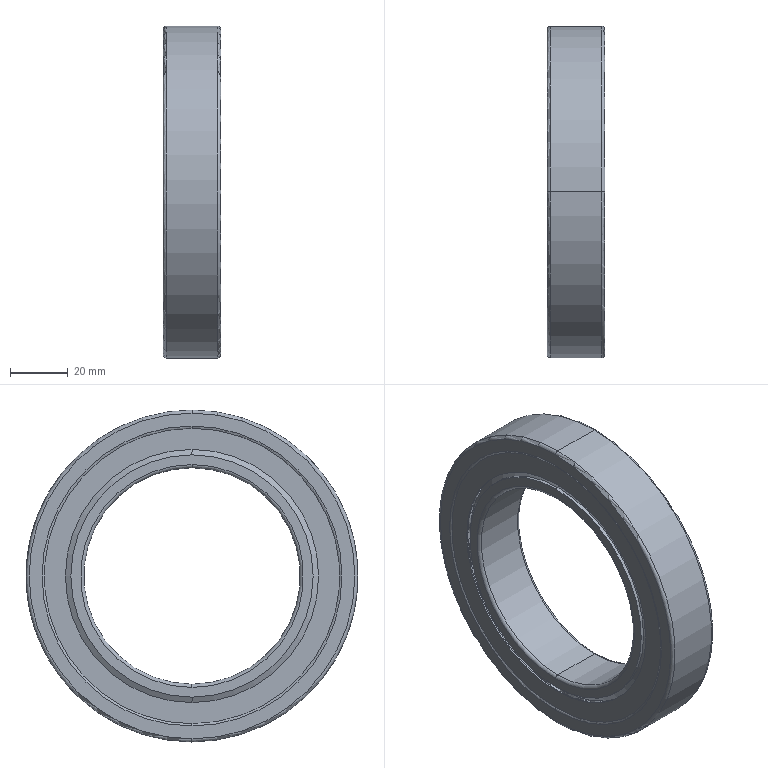Part | SolidWorks | features Revolution 5, CirPattern 2, RefAxis 1, RevCut 1 | 26 solids | 292 faces | box 20 x 115 x 115 mm | volume 89523 mm3 | cylinder 110 | sphere 100 | plane 56 | torus 22 | cone 4 | commonest cylinder face diameters 93 x47 97 x47 83.889 x4 88.333 x4 101.667 x4 75 x2